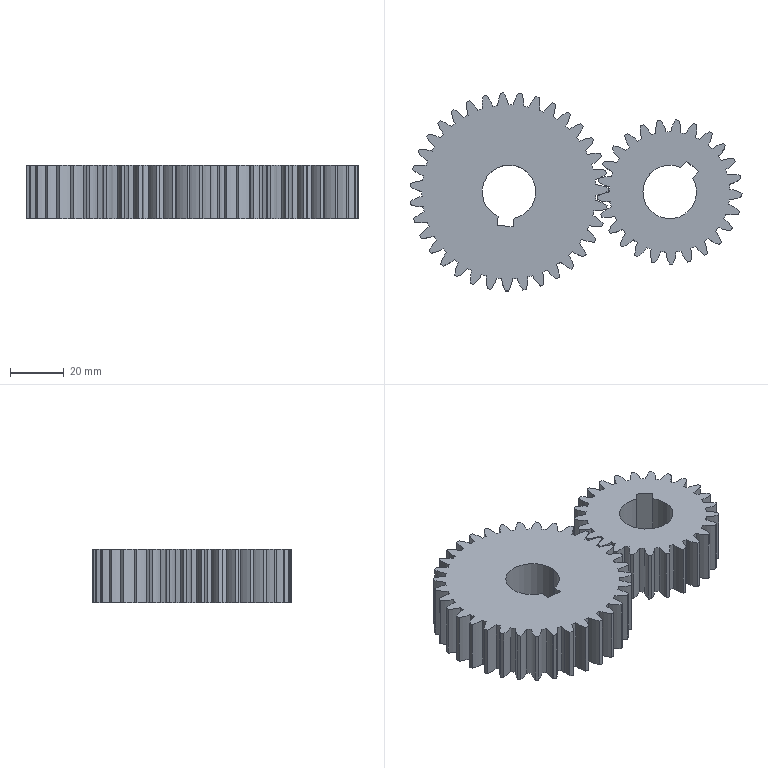Part | SolidWorks | features RefAxis 2 | 2 solids | 264 faces | box 123.948 x 73.952 x 20 mm | volume 100534 mm3 | cylinder 254 | plane 10 | commonest cylinder face diameters 28 x74 20 x60 64.998 x35 74 x35 44.998 x25 54 x25